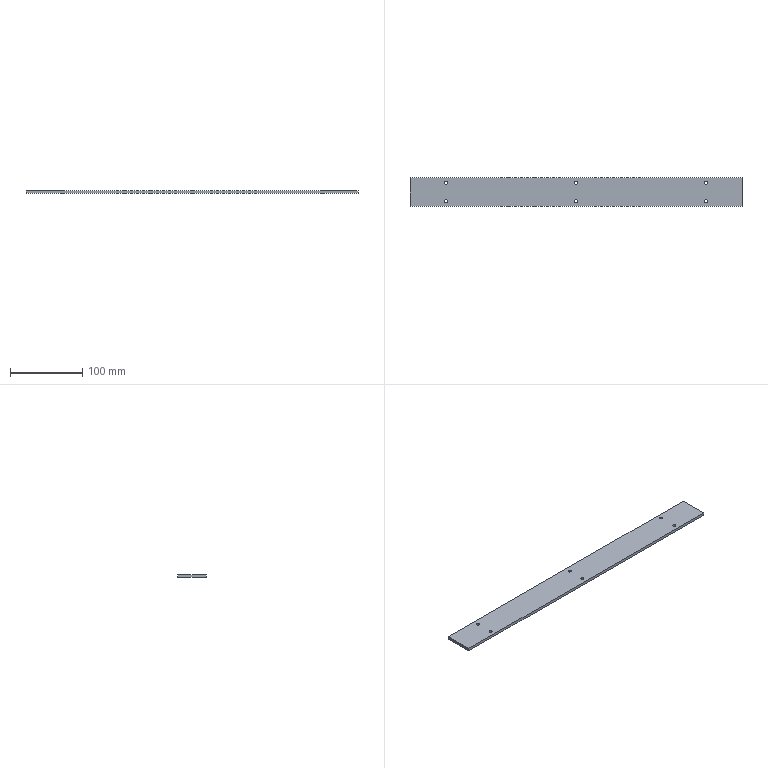Part | SolidWorks | features Extrusion 1, HoleWzd 1 | 1 solid | 18 faces | box 460 x 40 x 4 mm | volume 73267 mm3 | cylinder 12 | plane 6 | commonest cylinder face diameters 4.2 x12
STEP:
#1=CARTESIAN_POINT('',(-182.1,12.5,-2.));
#2=VERTEX_POINT('',#1);
#3=CARTESIAN_POINT('',(-177.9,12.5,-2.));
#4=VERTEX_POINT('',#3);
#5=CARTESIAN_POINT('',(-180.,12.5,-2.));
#6=DIRECTION('',(0.,0.,1.));
#7=DIRECTION('',(1.,0.,0.));
#8=AXIS2_PLACEMENT_3D('',#5,#6,#7);
#9=CIRCLE('',#8,2.1);
#10=EDGE_CURVE('',#2,#4,#9,.T.);
#11=ORIENTED_EDGE('',*,*,#10,.F.);
#12=CARTESIAN_POINT('',(-182.1,12.5,2.));
#13=VERTEX_POINT('',#12);
#14=CARTESIAN_POINT('',(-182.1,12.5,2.));
#15=DIRECTION('',(0.,0.,1.));
#16=VECTOR('',#15,1000.);
#17=LINE('',#14,#16);
#18=EDGE_CURVE('',#2,#13,#17,.T.);
#19=ORIENTED_EDGE('',*,*,#18,.T.);
#20=CARTESIAN_POINT('',(-177.9,12.5,2.));
#21=VERTEX_POINT('',#20);
#22=CARTESIAN_POINT('',(-180.,12.5,2.));
#23=DIRECTION('',(0.,0.,1.));
#24=DIRECTION('',(1.,0.,0.));
#25=AXIS2_PLACEMENT_3D('',#22,#23,#24);
#26=CIRCLE('',#25,2.1);
#27=EDGE_CURVE('',#13,#21,#26,.T.);
#28=ORIENTED_EDGE('',*,*,#27,.T.);
#29=CARTESIAN_POINT('',(-177.9,12.5,2.));
#30=DIRECTION('',(0.,0.,1.));
#31=VECTOR('',#30,1000.);
#32=LINE('',#29,#31);
#33=EDGE_CURVE('',#4,#21,#32,.T.);
#34=ORIENTED_EDGE('',*,*,#33,.F.);
#35=EDGE_LOOP('',(#11,#19,#28,#34));
#36=FACE_OUTER_BOUND('',#35,.T.);
#37=CARTESIAN_POINT('',(-180.,12.5,2.));
#38=DIRECTION('',(0.,0.,1.));
#39=DIRECTION('',(1.,0.,0.));
#40=AXIS2_PLACEMENT_3D('',#37,#38,#39);
#41=CYLINDRICAL_SURFACE('',#40,2.1);
#42=ADVANCED_FACE('',(#36),#41,.F.);
#43=CARTESIAN_POINT('',(-182.1,-12.5,-2.));
#44=VERTEX_POINT('',#43);
#45=CARTESIAN_POINT('',(-177.9,-12.5,-2.));
#46=VERTEX_POINT('',#45);
#47=CARTESIAN_POINT('',(-180.,-12.5,-2.));
#48=DIRECTION('',(0.,0.,1.));
#49=DIRECTION('',(1.,0.,0.));
#50=AXIS2_PLACEMENT_3D('',#47,#48,#49);
#51=CIRCLE('',#50,2.1);
#52=EDGE_CURVE('',#44,#46,#51,.T.);
#53=ORIENTED_EDGE('',*,*,#52,.F.);
#54=CARTESIAN_POINT('',(-182.1,-12.5,2.));
#55=VERTEX_POINT('',#54);
#56=CARTESIAN_POINT('',(-182.1,-12.5,2.));
#57=DIRECTION('',(0.,0.,1.));
#58=VECTOR('',#57,1000.);
#59=LINE('',#56,#58);
#60=EDGE_CURVE('',#44,#55,#59,.T.);
#61=ORIENTED_EDGE('',*,*,#60,.T.);
#62=CARTESIAN_POINT('',(-177.9,-12.5,2.));
#63=VERTEX_POINT('',#62);
#64=CARTESIAN_POINT('',(-180.,-12.5,2.));
#65=DIRECTION('',(0.,0.,1.));
#66=DIRECTION('',(1.,0.,0.));
#67=AXIS2_PLACEMENT_3D('',#64,#65,#66);
#68=CIRCLE('',#67,2.1);
#69=EDGE_CURVE('',#55,#63,#68,.T.);
#70=ORIENTED_EDGE('',*,*,#69,.T.);
#71=CARTESIAN_POINT('',(-177.9,-12.5,2.));
#72=DIRECTION('',(0.,0.,1.));
#73=VECTOR('',#72,1000.);
#74=LINE('',#71,#73);
#75=EDGE_CURVE('',#46,#63,#74,.T.);
#76=ORIENTED_EDGE('',*,*,#75,.F.);
#77=EDGE_LOOP('',(#53,#61,#70,#76));
#78=FACE_OUTER_BOUND('',#77,.T.);
#79=CARTESIAN_POINT('',(-180.,-12.5,2.));
#80=DIRECTION('',(0.,0.,1.));
#81=DIRECTION('',(1.,0.,0.));
#82=AXIS2_PLACEMENT_3D('',#79,#80,#81);
#83=CYLINDRICAL_SURFACE('',#82,2.1);
#84=ADVANCED_FACE('',(#78),#83,.F.);
#85=CARTESIAN_POINT('',(-2.1,12.5,-2.));
#86=VERTEX_POINT('',#85);
#87=CARTESIAN_POINT('',(2.1,12.5,-2.));
#88=VERTEX_POINT('',#87);
#89=CARTESIAN_POINT('',(0.,12.5,-2.));
#90=DIRECTION('',(0.,0.,1.));
#91=DIRECTION('',(1.,0.,0.));
#92=AXIS2_PLACEMENT_3D('',#89,#90,#91);
#93=CIRCLE('',#92,2.1);
#94=EDGE_CURVE('',#86,#88,#93,.T.);
#95=ORIENTED_EDGE('',*,*,#94,.F.);
#96=CARTESIAN_POINT('',(-2.1,12.5,2.));
#97=VERTEX_POINT('',#96);
#98=CARTESIAN_POINT('',(-2.1,12.5,2.));
#99=DIRECTION('',(0.,0.,1.));
#100=VECTOR('',#99,1000.);
#101=LINE('',#98,#100);
#102=EDGE_CURVE('',#86,#97,#101,.T.);
#103=ORIENTED_EDGE('',*,*,#102,.T.);
#104=CARTESIAN_POINT('',(2.1,12.5,2.));
#105=VERTEX_POINT('',#104);
#106=CARTESIAN_POINT('',(0.,12.5,2.));
#107=DIRECTION('',(0.,0.,1.));
#108=DIRECTION('',(1.,0.,0.));
#109=AXIS2_PLACEMENT_3D('',#106,#107,#108);
#110=CIRCLE('',#109,2.1);
#111=EDGE_CURVE('',#97,#105,#110,.T.);
#112=ORIENTED_EDGE('',*,*,#111,.T.);
#113=CARTESIAN_POINT('',(2.1,12.5,2.));
#114=DIRECTION('',(0.,0.,1.));
#115=VECTOR('',#114,1000.);
#116=LINE('',#113,#115);
#117=EDGE_CURVE('',#88,#105,#116,.T.);
#118=ORIENTED_EDGE('',*,*,#117,.F.);
#119=EDGE_LOOP('',(#95,#103,#112,#118));
#120=FACE_OUTER_BOUND('',#119,.T.);
#121=CARTESIAN_POINT('',(0.,12.5,2.));
#122=DIRECTION('',(0.,0.,1.));
#123=DIRECTION('',(1.,0.,0.));
#124=AXIS2_PLACEMENT_3D('',#121,#122,#123);
#125=CYLINDRICAL_SURFACE('',#124,2.1);
#126=ADVANCED_FACE('',(#120),#125,.F.);
#127=CARTESIAN_POINT('',(-2.1,-12.5,-2.));
#128=VERTEX_POINT('',#127);
#129=CARTESIAN_POINT('',(2.1,-12.5,-2.));
#130=VERTEX_POINT('',#129);
#131=CARTESIAN_POINT('',(0.,-12.5,-2.));
#132=DIRECTION('',(0.,0.,1.));
#133=DIRECTION('',(1.,0.,0.));
#134=AXIS2_PLACEMENT_3D('',#131,#132,#133);
#135=CIRCLE('',#134,2.1);
#136=EDGE_CURVE('',#128,#130,#135,.T.);
#137=ORIENTED_EDGE('',*,*,#136,.F.);
#138=CARTESIAN_POINT('',(-2.1,-12.5,2.));
#139=VERTEX_POINT('',#138);
#140=CARTESIAN_POINT('',(-2.1,-12.5,2.));
#141=DIRECTION('',(0.,0.,1.));
#142=VECTOR('',#141,1000.);
#143=LINE('',#140,#142);
#144=EDGE_CURVE('',#128,#139,#143,.T.);
#145=ORIENTED_EDGE('',*,*,#144,.T.);
#146=CARTESIAN_POINT('',(2.1,-12.5,2.));
#147=VERTEX_POINT('',#146);
#148=CARTESIAN_POINT('',(0.,-12.5,2.));
#149=DIRECTION('',(0.,0.,1.));
#150=DIRECTION('',(1.,0.,0.));
#151=AXIS2_PLACEMENT_3D('',#148,#149,#150);
#152=CIRCLE('',#151,2.1);
#153=EDGE_CURVE('',#139,#147,#152,.T.);
#154=ORIENTED_EDGE('',*,*,#153,.T.);
#155=CARTESIAN_POINT('',(2.1,-12.5,2.));
#156=DIRECTION('',(0.,0.,1.));
#157=VECTOR('',#156,1000.);
#158=LINE('',#155,#157);
#159=EDGE_CURVE('',#130,#147,#158,.T.);
#160=ORIENTED_EDGE('',*,*,#159,.F.);
#161=EDGE_LOOP('',(#137,#145,#154,#160));
#162=FACE_OUTER_BOUND('',#161,.T.);
#163=CARTESIAN_POINT('',(0.,-12.5,2.));
#164=DIRECTION('',(0.,0.,1.));
#165=DIRECTION('',(1.,0.,0.));
#166=AXIS2_PLACEMENT_3D('',#163,#164,#165);
#167=CYLINDRICAL_SURFACE('',#166,2.1);
#168=ADVANCED_FACE('',(#162),#167,.F.);
#169=CARTESIAN_POINT('',(177.9,12.5,-2.));
#170=VERTEX_POINT('',#169);
#171=CARTESIAN_POINT('',(182.1,12.5,-2.));
#172=VERTEX_POINT('',#171);
#173=CARTESIAN_POINT('',(180.,12.5,-2.));
#174=DIRECTION('',(0.,0.,1.));
#175=DIRECTION('',(1.,0.,0.));
#176=AXIS2_PLACEMENT_3D('',#173,#174,#175);
#177=CIRCLE('',#176,2.1);
#178=EDGE_CURVE('',#170,#172,#177,.T.);
#179=ORIENTED_EDGE('',*,*,#178,.F.);
#180=CARTESIAN_POINT('',(177.9,12.5,2.));
#181=VERTEX_POINT('',#180);
#182=CARTESIAN_POINT('',(177.9,12.5,2.));
#183=DIRECTION('',(0.,0.,1.));
#184=VECTOR('',#183,1000.);
#185=LINE('',#182,#184);
#186=EDGE_CURVE('',#170,#181,#185,.T.);
#187=ORIENTED_EDGE('',*,*,#186,.T.);
#188=CARTESIAN_POINT('',(182.1,12.5,2.));
#189=VERTEX_POINT('',#188);
#190=CARTESIAN_POINT('',(180.,12.5,2.));
#191=DIRECTION('',(0.,0.,1.));
#192=DIRECTION('',(1.,0.,0.));
#193=AXIS2_PLACEMENT_3D('',#190,#191,#192);
#194=CIRCLE('',#193,2.1);
#195=EDGE_CURVE('',#181,#189,#194,.T.);
#196=ORIENTED_EDGE('',*,*,#195,.T.);
#197=CARTESIAN_POINT('',(182.1,12.5,2.));
#198=DIRECTION('',(0.,0.,1.));
#199=VECTOR('',#198,1000.);
#200=LINE('',#197,#199);
#201=EDGE_CURVE('',#172,#189,#200,.T.);
#202=ORIENTED_EDGE('',*,*,#201,.F.);
#203=EDGE_LOOP('',(#179,#187,#196,#202));
#204=FACE_OUTER_BOUND('',#203,.T.);
#205=CARTESIAN_POINT('',(180.,12.5,2.));
#206=DIRECTION('',(0.,0.,1.));
#207=DIRECTION('',(1.,0.,0.));
#208=AXIS2_PLACEMENT_3D('',#205,#206,#207);
#209=CYLINDRICAL_SURFACE('',#208,2.1);
#210=ADVANCED_FACE('',(#204),#209,.F.);
#211=CARTESIAN_POINT('',(177.9,-12.5,-2.));
#212=VERTEX_POINT('',#211);
#213=CARTESIAN_POINT('',(182.1,-12.5,-2.));
#214=VERTEX_POINT('',#213);
#215=CARTESIAN_POINT('',(180.,-12.5,-2.));
#216=DIRECTION('',(0.,0.,1.));
#217=DIRECTION('',(1.,0.,0.));
#218=AXIS2_PLACEMENT_3D('',#215,#216,#217);
#219=CIRCLE('',#218,2.1);
#220=EDGE_CURVE('',#212,#214,#219,.T.);
#221=ORIENTED_EDGE('',*,*,#220,.F.);
#222=CARTESIAN_POINT('',(177.9,-12.5,2.));
#223=VERTEX_POINT('',#222);
#224=CARTESIAN_POINT('',(177.9,-12.5,2.));
#225=DIRECTION('',(0.,0.,1.));
#226=VECTOR('',#225,1000.);
#227=LINE('',#224,#226);
#228=EDGE_CURVE('',#212,#223,#227,.T.);
#229=ORIENTED_EDGE('',*,*,#228,.T.);
#230=CARTESIAN_POINT('',(182.1,-12.5,2.));
#231=VERTEX_POINT('',#230);
#232=CARTESIAN_POINT('',(180.,-12.5,2.));
#233=DIRECTION('',(0.,0.,1.));
#234=DIRECTION('',(1.,0.,0.));
#235=AXIS2_PLACEMENT_3D('',#232,#233,#234);
#236=CIRCLE('',#235,2.1);
#237=EDGE_CURVE('',#223,#231,#236,.T.);
#238=ORIENTED_EDGE('',*,*,#237,.T.);
#239=CARTESIAN_POINT('',(182.1,-12.5,2.));
#240=DIRECTION('',(0.,0.,1.));
#241=VECTOR('',#240,1000.);
#242=LINE('',#239,#241);
#243=EDGE_CURVE('',#214,#231,#242,.T.);
#244=ORIENTED_EDGE('',*,*,#243,.F.);
#245=EDGE_LOOP('',(#221,#229,#238,#244));
#246=FACE_OUTER_BOUND('',#245,.T.);
#247=CARTESIAN_POINT('',(180.,-12.5,2.));
#248=DIRECTION('',(0.,0.,1.));
#249=DIRECTION('',(1.,0.,0.));
#250=AXIS2_PLACEMENT_3D('',#247,#248,#249);
#251=CYLINDRICAL_SURFACE('',#250,2.1);
#252=ADVANCED_FACE('',(#246),#251,.F.);
#253=CARTESIAN_POINT('',(230.,-20.,-2.));
#254=VERTEX_POINT('',#253);
#255=CARTESIAN_POINT('',(230.,20.,-2.));
#256=VERTEX_POINT('',#255);
#257=CARTESIAN_POINT('',(230.,20.,-2.));
#258=DIRECTION('',(0.,1.,0.));
#259=VECTOR('',#258,1000.);
#260=LINE('',#257,#259);
#261=EDGE_CURVE('',#254,#256,#260,.T.);
#262=ORIENTED_EDGE('',*,*,#261,.T.);
#263=CARTESIAN_POINT('',(230.,20.,2.));
#264=VERTEX_POINT('',#263);
#265=CARTESIAN_POINT('',(230.,20.,2.));
#266=DIRECTION('',(0.,0.,-1.));
#267=VECTOR('',#266,1000.);
#268=LINE('',#265,#267);
#269=EDGE_CURVE('',#264,#256,#268,.T.);
#270=ORIENTED_EDGE('',*,*,#269,.F.);
#271=CARTESIAN_POINT('',(230.,-20.,2.));
#272=VERTEX_POINT('',#271);
#273=CARTESIAN_POINT('',(230.,20.,2.));
#274=DIRECTION('',(0.,1.,0.));
#275=VECTOR('',#274,1000.);
#276=LINE('',#273,#275);
#277=EDGE_CURVE('',#272,#264,#276,.T.);
#278=ORIENTED_EDGE('',*,*,#277,.F.);
#279=CARTESIAN_POINT('',(230.,-20.,2.));
#280=DIRECTION('',(0.,0.,-1.));
#281=VECTOR('',#280,1000.);
#282=LINE('',#279,#281);
#283=EDGE_CURVE('',#272,#254,#282,.T.);
#284=ORIENTED_EDGE('',*,*,#283,.T.);
#285=EDGE_LOOP('',(#262,#270,#278,#284));
#286=FACE_OUTER_BOUND('',#285,.T.);
#287=CARTESIAN_POINT('',(230.,20.,2.));
#288=DIRECTION('',(-1.,0.,0.));
#289=DIRECTION('',(0.,-1.,0.));
#290=AXIS2_PLACEMENT_3D('',#287,#288,#289);
#291=PLANE('',#290);
#292=ADVANCED_FACE('',(#286),#291,.F.);
#293=CARTESIAN_POINT('',(-230.,20.,-2.));
#294=VERTEX_POINT('',#293);
#295=CARTESIAN_POINT('',(-230.,20.,-2.));
#296=DIRECTION('',(-1.,0.,0.));
#297=VECTOR('',#296,1000.);
#298=LINE('',#295,#297);
#299=EDGE_CURVE('',#256,#294,#298,.T.);
#300=ORIENTED_EDGE('',*,*,#299,.T.);
#301=CARTESIAN_POINT('',(-230.,20.,2.));
#302=VERTEX_POINT('',#301);
#303=CARTESIAN_POINT('',(-230.,20.,2.));
#304=DIRECTION('',(0.,0.,-1.));
#305=VECTOR('',#304,1000.);
#306=LINE('',#303,#305);
#307=EDGE_CURVE('',#302,#294,#306,.T.);
#308=ORIENTED_EDGE('',*,*,#307,.F.);
#309=CARTESIAN_POINT('',(-230.,20.,2.));
#310=DIRECTION('',(-1.,0.,0.));
#311=VECTOR('',#310,1000.);
#312=LINE('',#309,#311);
#313=EDGE_CURVE('',#264,#302,#312,.T.);
#314=ORIENTED_EDGE('',*,*,#313,.F.);
#315=ORIENTED_EDGE('',*,*,#269,.T.);
#316=EDGE_LOOP('',(#300,#308,#314,#315));
#317=FACE_OUTER_BOUND('',#316,.T.);
#318=CARTESIAN_POINT('',(-230.,20.,2.));
#319=DIRECTION('',(0.,-1.,0.));
#320=DIRECTION('',(0.,0.,-1.));
#321=AXIS2_PLACEMENT_3D('',#318,#319,#320);
#322=PLANE('',#321);
#323=ADVANCED_FACE('',(#317),#322,.F.);
#324=CARTESIAN_POINT('',(-230.,-20.,-2.));
#325=VERTEX_POINT('',#324);
#326=CARTESIAN_POINT('',(-230.,20.,-2.));
#327=DIRECTION('',(0.,-1.,0.));
#328=VECTOR('',#327,1000.);
#329=LINE('',#326,#328);
#330=EDGE_CURVE('',#294,#325,#329,.T.);
#331=ORIENTED_EDGE('',*,*,#330,.T.);
#332=CARTESIAN_POINT('',(-230.,-20.,2.));
#333=VERTEX_POINT('',#332);
#334=CARTESIAN_POINT('',(-230.,-20.,2.));
#335=DIRECTION('',(0.,0.,-1.));
#336=VECTOR('',#335,1000.);
#337=LINE('',#334,#336);
#338=EDGE_CURVE('',#333,#325,#337,.T.);
#339=ORIENTED_EDGE('',*,*,#338,.F.);
#340=CARTESIAN_POINT('',(-230.,20.,2.));
#341=DIRECTION('',(0.,-1.,0.));
#342=VECTOR('',#341,1000.);
#343=LINE('',#340,#342);
#344=EDGE_CURVE('',#302,#333,#343,.T.);
#345=ORIENTED_EDGE('',*,*,#344,.F.);
#346=ORIENTED_EDGE('',*,*,#307,.T.);
#347=EDGE_LOOP('',(#331,#339,#345,#346));
#348=FACE_OUTER_BOUND('',#347,.T.);
#349=CARTESIAN_POINT('',(-230.,20.,2.));
#350=DIRECTION('',(1.,0.,0.));
#351=DIRECTION('',(0.,0.,-1.));
#352=AXIS2_PLACEMENT_3D('',#349,#350,#351);
#353=PLANE('',#352);
#354=ADVANCED_FACE('',(#348),#353,.F.);
#355=CARTESIAN_POINT('',(-230.,-20.,-2.));
#356=DIRECTION('',(1.,0.,0.));
#357=VECTOR('',#356,1000.);
#358=LINE('',#355,#357);
#359=EDGE_CURVE('',#325,#254,#358,.T.);
#360=ORIENTED_EDGE('',*,*,#359,.T.);
#361=ORIENTED_EDGE('',*,*,#283,.F.);
#362=CARTESIAN_POINT('',(-230.,-20.,2.));
#363=DIRECTION('',(1.,0.,0.));
#364=VECTOR('',#363,1000.);
#365=LINE('',#362,#364);
#366=EDGE_CURVE('',#333,#272,#365,.T.);
#367=ORIENTED_EDGE('',*,*,#366,.F.);
#368=ORIENTED_EDGE('',*,*,#338,.T.);
#369=EDGE_LOOP('',(#360,#361,#367,#368));
#370=FACE_OUTER_BOUND('',#369,.T.);
#371=CARTESIAN_POINT('',(-230.,-20.,2.));
#372=DIRECTION('',(0.,1.,0.));
#373=DIRECTION('',(0.,0.,1.));
#374=AXIS2_PLACEMENT_3D('',#371,#372,#373);
#375=PLANE('',#374);
#376=ADVANCED_FACE('',(#370),#375,.F.);
#377=CARTESIAN_POINT('',(-180.,12.5,2.));
#378=DIRECTION('',(0.,0.,1.));
#379=DIRECTION('',(1.,0.,0.));
#380=AXIS2_PLACEMENT_3D('',#377,#378,#379);
#381=CIRCLE('',#380,2.1);
#382=EDGE_CURVE('',#21,#13,#381,.T.);
#383=ORIENTED_EDGE('',*,*,#382,.F.);
#384=ORIENTED_EDGE('',*,*,#27,.F.);
#385=EDGE_LOOP('',(#383,#384));
#386=FACE_BOUND('',#385,.T.);
#387=CARTESIAN_POINT('',(-180.,-12.5,2.));
#388=DIRECTION('',(0.,0.,1.));
#389=DIRECTION('',(1.,0.,0.));
#390=AXIS2_PLACEMENT_3D('',#387,#388,#389);
#391=CIRCLE('',#390,2.1);
#392=EDGE_CURVE('',#63,#55,#391,.T.);
#393=ORIENTED_EDGE('',*,*,#392,.F.);
#394=ORIENTED_EDGE('',*,*,#69,.F.);
#395=EDGE_LOOP('',(#393,#394));
#396=FACE_BOUND('',#395,.T.);
#397=CARTESIAN_POINT('',(0.,12.5,2.));
#398=DIRECTION('',(0.,0.,1.));
#399=DIRECTION('',(1.,0.,0.));
#400=AXIS2_PLACEMENT_3D('',#397,#398,#399);
#401=CIRCLE('',#400,2.1);
#402=EDGE_CURVE('',#105,#97,#401,.T.);
#403=ORIENTED_EDGE('',*,*,#402,.F.);
#404=ORIENTED_EDGE('',*,*,#111,.F.);
#405=EDGE_LOOP('',(#403,#404));
#406=FACE_BOUND('',#405,.T.);
#407=CARTESIAN_POINT('',(0.,-12.5,2.));
#408=DIRECTION('',(0.,0.,1.));
#409=DIRECTION('',(1.,0.,0.));
#410=AXIS2_PLACEMENT_3D('',#407,#408,#409);
#411=CIRCLE('',#410,2.1);
#412=EDGE_CURVE('',#147,#139,#411,.T.);
#413=ORIENTED_EDGE('',*,*,#412,.F.);
#414=ORIENTED_EDGE('',*,*,#153,.F.);
#415=EDGE_LOOP('',(#413,#414));
#416=FACE_BOUND('',#415,.T.);
#417=CARTESIAN_POINT('',(180.,12.5,2.));
#418=DIRECTION('',(0.,0.,1.));
#419=DIRECTION('',(1.,0.,0.));
#420=AXIS2_PLACEMENT_3D('',#417,#418,#419);
#421=CIRCLE('',#420,2.1);
#422=EDGE_CURVE('',#189,#181,#421,.T.);
#423=ORIENTED_EDGE('',*,*,#422,.F.);
#424=ORIENTED_EDGE('',*,*,#195,.F.);
#425=EDGE_LOOP('',(#423,#424));
#426=FACE_BOUND('',#425,.T.);
#427=CARTESIAN_POINT('',(180.,-12.5,2.));
#428=DIRECTION('',(0.,0.,1.));
#429=DIRECTION('',(1.,0.,0.));
#430=AXIS2_PLACEMENT_3D('',#427,#428,#429);
#431=CIRCLE('',#430,2.1);
#432=EDGE_CURVE('',#231,#223,#431,.T.);
#433=ORIENTED_EDGE('',*,*,#432,.F.);
#434=ORIENTED_EDGE('',*,*,#237,.F.);
#435=EDGE_LOOP('',(#433,#434));
#436=FACE_BOUND('',#435,.T.);
#437=ORIENTED_EDGE('',*,*,#277,.T.);
#438=ORIENTED_EDGE('',*,*,#313,.T.);
#439=ORIENTED_EDGE('',*,*,#344,.T.);
#440=ORIENTED_EDGE('',*,*,#366,.T.);
#441=EDGE_LOOP('',(#437,#438,#439,#440));
#442=FACE_OUTER_BOUND('',#441,.T.);
#443=CARTESIAN_POINT('',(0.,0.,2.));
#444=DIRECTION('',(0.,0.,1.));
#445=DIRECTION('',(1.,0.,0.));
#446=AXIS2_PLACEMENT_3D('',#443,#444,#445);
#447=PLANE('',#446);
#448=ADVANCED_FACE('',(#386,#396,#406,#416,#426,#436,#442),#447,.T.);
#449=CARTESIAN_POINT('',(-180.,12.5,-2.));
#450=DIRECTION('',(0.,0.,1.));
#451=DIRECTION('',(1.,0.,0.));
#452=AXIS2_PLACEMENT_3D('',#449,#450,#451);
#453=CIRCLE('',#452,2.1);
#454=EDGE_CURVE('',#4,#2,#453,.T.);
#455=ORIENTED_EDGE('',*,*,#454,.T.);
#456=ORIENTED_EDGE('',*,*,#10,.T.);
#457=EDGE_LOOP('',(#455,#456));
#458=FACE_BOUND('',#457,.T.);
#459=CARTESIAN_POINT('',(-180.,-12.5,-2.));
#460=DIRECTION('',(0.,0.,1.));
#461=DIRECTION('',(1.,0.,0.));
#462=AXIS2_PLACEMENT_3D('',#459,#460,#461);
#463=CIRCLE('',#462,2.1);
#464=EDGE_CURVE('',#46,#44,#463,.T.);
#465=ORIENTED_EDGE('',*,*,#464,.T.);
#466=ORIENTED_EDGE('',*,*,#52,.T.);
#467=EDGE_LOOP('',(#465,#466));
#468=FACE_BOUND('',#467,.T.);
#469=CARTESIAN_POINT('',(0.,12.5,-2.));
#470=DIRECTION('',(0.,0.,1.));
#471=DIRECTION('',(1.,0.,0.));
#472=AXIS2_PLACEMENT_3D('',#469,#470,#471);
#473=CIRCLE('',#472,2.1);
#474=EDGE_CURVE('',#88,#86,#473,.T.);
#475=ORIENTED_EDGE('',*,*,#474,.T.);
#476=ORIENTED_EDGE('',*,*,#94,.T.);
#477=EDGE_LOOP('',(#475,#476));
#478=FACE_BOUND('',#477,.T.);
#479=CARTESIAN_POINT('',(0.,-12.5,-2.));
#480=DIRECTION('',(0.,0.,1.));
#481=DIRECTION('',(1.,0.,0.));
#482=AXIS2_PLACEMENT_3D('',#479,#480,#481);
#483=CIRCLE('',#482,2.1);
#484=EDGE_CURVE('',#130,#128,#483,.T.);
#485=ORIENTED_EDGE('',*,*,#484,.T.);
#486=ORIENTED_EDGE('',*,*,#136,.T.);
#487=EDGE_LOOP('',(#485,#486));
#488=FACE_BOUND('',#487,.T.);
#489=CARTESIAN_POINT('',(180.,12.5,-2.));
#490=DIRECTION('',(0.,0.,1.));
#491=DIRECTION('',(1.,0.,0.));
#492=AXIS2_PLACEMENT_3D('',#489,#490,#491);
#493=CIRCLE('',#492,2.1);
#494=EDGE_CURVE('',#172,#170,#493,.T.);
#495=ORIENTED_EDGE('',*,*,#494,.T.);
#496=ORIENTED_EDGE('',*,*,#178,.T.);
#497=EDGE_LOOP('',(#495,#496));
#498=FACE_BOUND('',#497,.T.);
#499=CARTESIAN_POINT('',(180.,-12.5,-2.));
#500=DIRECTION('',(0.,0.,1.));
#501=DIRECTION('',(1.,0.,0.));
#502=AXIS2_PLACEMENT_3D('',#499,#500,#501);
#503=CIRCLE('',#502,2.1);
#504=EDGE_CURVE('',#214,#212,#503,.T.);
#505=ORIENTED_EDGE('',*,*,#504,.T.);
#506=ORIENTED_EDGE('',*,*,#220,.T.);
#507=EDGE_LOOP('',(#505,#506));
#508=FACE_BOUND('',#507,.T.);
#509=ORIENTED_EDGE('',*,*,#261,.F.);
#510=ORIENTED_EDGE('',*,*,#359,.F.);
#511=ORIENTED_EDGE('',*,*,#330,.F.);
#512=ORIENTED_EDGE('',*,*,#299,.F.);
#513=EDGE_LOOP('',(#509,#510,#511,#512));
#514=FACE_OUTER_BOUND('',#513,.T.);
#515=CARTESIAN_POINT('',(0.,0.,-2.));
#516=DIRECTION('',(0.,0.,1.));
#517=DIRECTION('',(1.,0.,0.));
#518=AXIS2_PLACEMENT_3D('',#515,#516,#517);
#519=PLANE('',#518);
#520=ADVANCED_FACE('',(#458,#468,#478,#488,#498,#508,#514),#519,.F.);
#521=ORIENTED_EDGE('',*,*,#228,.F.);
#522=ORIENTED_EDGE('',*,*,#504,.F.);
#523=ORIENTED_EDGE('',*,*,#243,.T.);
#524=ORIENTED_EDGE('',*,*,#432,.T.);
#525=EDGE_LOOP('',(#521,#522,#523,#524));
#526=FACE_OUTER_BOUND('',#525,.T.);
#527=CARTESIAN_POINT('',(180.,-12.5,2.));
#528=DIRECTION('',(0.,0.,1.));
#529=DIRECTION('',(1.,0.,0.));
#530=AXIS2_PLACEMENT_3D('',#527,#528,#529);
#531=CYLINDRICAL_SURFACE('',#530,2.1);
#532=ADVANCED_FACE('',(#526),#531,.F.);
#533=ORIENTED_EDGE('',*,*,#186,.F.);
#534=ORIENTED_EDGE('',*,*,#494,.F.);
#535=ORIENTED_EDGE('',*,*,#201,.T.);
#536=ORIENTED_EDGE('',*,*,#422,.T.);
#537=EDGE_LOOP('',(#533,#534,#535,#536));
#538=FACE_OUTER_BOUND('',#537,.T.);
#539=CARTESIAN_POINT('',(180.,12.5,2.));
#540=DIRECTION('',(0.,0.,1.));
#541=DIRECTION('',(1.,0.,0.));
#542=AXIS2_PLACEMENT_3D('',#539,#540,#541);
#543=CYLINDRICAL_SURFACE('',#542,2.1);
#544=ADVANCED_FACE('',(#538),#543,.F.);
#545=ORIENTED_EDGE('',*,*,#144,.F.);
#546=ORIENTED_EDGE('',*,*,#484,.F.);
#547=ORIENTED_EDGE('',*,*,#159,.T.);
#548=ORIENTED_EDGE('',*,*,#412,.T.);
#549=EDGE_LOOP('',(#545,#546,#547,#548));
#550=FACE_OUTER_BOUND('',#549,.T.);
#551=CARTESIAN_POINT('',(0.,-12.5,2.));
#552=DIRECTION('',(0.,0.,1.));
#553=DIRECTION('',(1.,0.,0.));
#554=AXIS2_PLACEMENT_3D('',#551,#552,#553);
#555=CYLINDRICAL_SURFACE('',#554,2.1);
#556=ADVANCED_FACE('',(#550),#555,.F.);
#557=ORIENTED_EDGE('',*,*,#102,.F.);
#558=ORIENTED_EDGE('',*,*,#474,.F.);
#559=ORIENTED_EDGE('',*,*,#117,.T.);
#560=ORIENTED_EDGE('',*,*,#402,.T.);
#561=EDGE_LOOP('',(#557,#558,#559,#560));
#562=FACE_OUTER_BOUND('',#561,.T.);
#563=CARTESIAN_POINT('',(0.,12.5,2.));
#564=DIRECTION('',(0.,0.,1.));
#565=DIRECTION('',(1.,0.,0.));
#566=AXIS2_PLACEMENT_3D('',#563,#564,#565);
#567=CYLINDRICAL_SURFACE('',#566,2.1);
#568=ADVANCED_FACE('',(#562),#567,.F.);
#569=ORIENTED_EDGE('',*,*,#60,.F.);
#570=ORIENTED_EDGE('',*,*,#464,.F.);
#571=ORIENTED_EDGE('',*,*,#75,.T.);
#572=ORIENTED_EDGE('',*,*,#392,.T.);
#573=EDGE_LOOP('',(#569,#570,#571,#572));
#574=FACE_OUTER_BOUND('',#573,.T.);
#575=CARTESIAN_POINT('',(-180.,-12.5,2.));
#576=DIRECTION('',(0.,0.,1.));
#577=DIRECTION('',(1.,0.,0.));
#578=AXIS2_PLACEMENT_3D('',#575,#576,#577);
#579=CYLINDRICAL_SURFACE('',#578,2.1);
#580=ADVANCED_FACE('',(#574),#579,.F.);
#581=ORIENTED_EDGE('',*,*,#18,.F.);
#582=ORIENTED_EDGE('',*,*,#454,.F.);
#583=ORIENTED_EDGE('',*,*,#33,.T.);
#584=ORIENTED_EDGE('',*,*,#382,.T.);
#585=EDGE_LOOP('',(#581,#582,#583,#584));
#586=FACE_OUTER_BOUND('',#585,.T.);
#587=CARTESIAN_POINT('',(-180.,12.5,2.));
#588=DIRECTION('',(0.,0.,1.));
#589=DIRECTION('',(1.,0.,0.));
#590=AXIS2_PLACEMENT_3D('',#587,#588,#589);
#591=CYLINDRICAL_SURFACE('',#590,2.1);
#592=ADVANCED_FACE('',(#586),#591,.F.);
#593=CLOSED_SHELL('',(#42,#84,#126,#168,#210,#252,#292,#323,#354,#376,#448,#520,#532,#544,#556,#568,#580,#592));
#594=MANIFOLD_SOLID_BREP('',#593);
#595=CARTESIAN_POINT('',(0.,0.,0.));
#596=DIRECTION('',(0.,0.,1.));
#597=DIRECTION('',(1.,0.,0.));
#598=AXIS2_PLACEMENT_3D('',#595,#596,#597);
#599=(LENGTH_UNIT()NAMED_UNIT(*)SI_UNIT(.MILLI.,.METRE.));
#600=UNCERTAINTY_MEASURE_WITH_UNIT(LENGTH_MEASURE(0.00001),#599,'','');
#601=(NAMED_UNIT(*)PLANE_ANGLE_UNIT()SI_UNIT($,.RADIAN.));
#602=(NAMED_UNIT(*)SI_UNIT($,.STERADIAN.)SOLID_ANGLE_UNIT());
#603=(GEOMETRIC_REPRESENTATION_CONTEXT(3)GLOBAL_UNCERTAINTY_ASSIGNED_CONTEXT((#600))GLOBAL_UNIT_ASSIGNED_CONTEXT((#599,#601,#602))REPRESENTATION_CONTEXT('',''));
#604=ADVANCED_BREP_SHAPE_REPRESENTATION('',(#594,#598),#603);